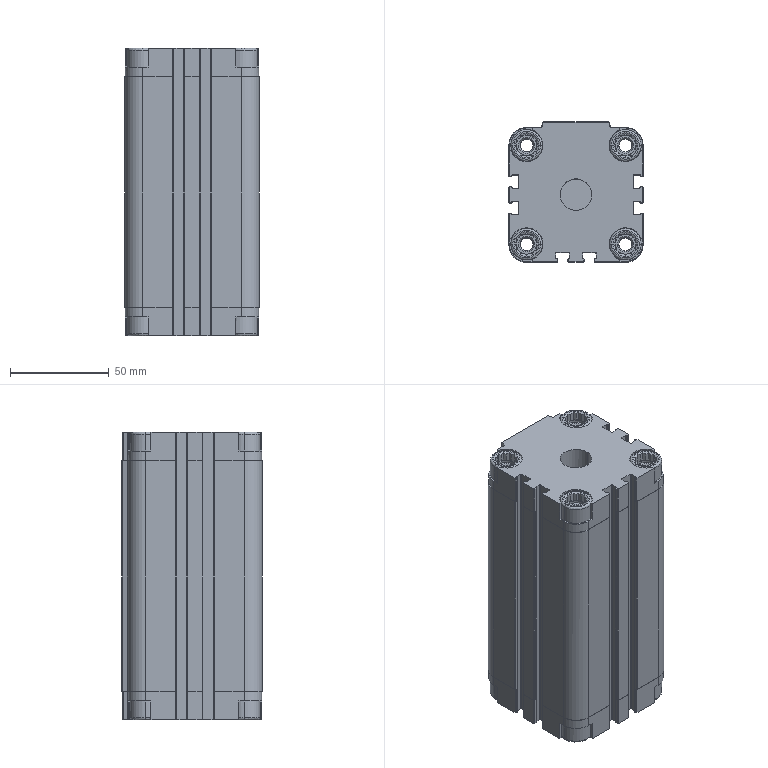Part | SolidWorks | 1 solid | 685 faces | box 68 x 71 x 145.5 mm | volume 391762 mm3 | plane 409 | cylinder 218 | cone 42 | torus 16 | commonest cylinder face diameters 0.8 x72 0.4 x48 16 x18 6.647 x16 10.2 x16 0.6 x12